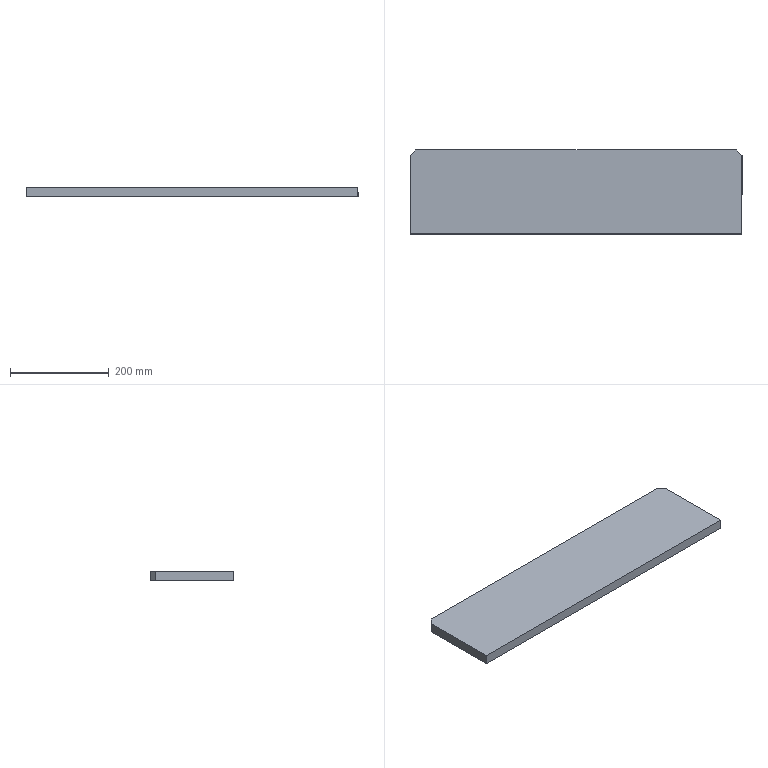Part | SolidWorks | features Chamfer 1, FlatPattern 1, SMBaseFlange 1, SheetMetal 1 | 1 solid | 8 faces | box 672 x 170 x 20 mm | volume 2281920 mm3 | plane 8
STEP:
#1=CARTESIAN_POINT('',(0.,158.,0.));
#2=VERTEX_POINT('',#1);
#3=CARTESIAN_POINT('',(0.,0.,0.));
#4=VERTEX_POINT('',#3);
#5=CARTESIAN_POINT('',(0.,0.,0.));
#6=DIRECTION('',(0.,-1.,0.));
#7=VECTOR('',#6,1000.);
#8=LINE('',#5,#7);
#9=EDGE_CURVE('',#2,#4,#8,.T.);
#10=ORIENTED_EDGE('',*,*,#9,.F.);
#11=CARTESIAN_POINT('',(0.,158.,-20.));
#12=VERTEX_POINT('',#11);
#13=CARTESIAN_POINT('',(0.,158.,-20.));
#14=DIRECTION('',(0.,0.,-1.));
#15=VECTOR('',#14,1000.);
#16=LINE('',#13,#15);
#17=EDGE_CURVE('',#2,#12,#16,.T.);
#18=ORIENTED_EDGE('',*,*,#17,.T.);
#19=CARTESIAN_POINT('',(0.,0.,-20.));
#20=VERTEX_POINT('',#19);
#21=CARTESIAN_POINT('',(0.,0.,-20.));
#22=DIRECTION('',(0.,-1.,0.));
#23=VECTOR('',#22,1000.);
#24=LINE('',#21,#23);
#25=EDGE_CURVE('',#12,#20,#24,.T.);
#26=ORIENTED_EDGE('',*,*,#25,.T.);
#27=CARTESIAN_POINT('',(0.,0.,-20.));
#28=DIRECTION('',(0.,0.,1.));
#29=VECTOR('',#28,1000.);
#30=LINE('',#27,#29);
#31=EDGE_CURVE('',#20,#4,#30,.T.);
#32=ORIENTED_EDGE('',*,*,#31,.T.);
#33=EDGE_LOOP('',(#10,#18,#26,#32));
#34=FACE_OUTER_BOUND('',#33,.T.);
#35=CARTESIAN_POINT('',(0.,0.,-20.));
#36=DIRECTION('',(-1.,0.,0.));
#37=DIRECTION('',(0.,0.,1.));
#38=AXIS2_PLACEMENT_3D('',#35,#36,#37);
#39=PLANE('',#38);
#40=ADVANCED_FACE('',(#34),#39,.T.);
#41=CARTESIAN_POINT('',(660.,170.,0.));
#42=VERTEX_POINT('',#41);
#43=CARTESIAN_POINT('',(12.,170.,0.));
#44=VERTEX_POINT('',#43);
#45=CARTESIAN_POINT('',(0.,170.,0.));
#46=DIRECTION('',(-1.,0.,0.));
#47=VECTOR('',#46,1000.);
#48=LINE('',#45,#47);
#49=EDGE_CURVE('',#42,#44,#48,.T.);
#50=ORIENTED_EDGE('',*,*,#49,.F.);
#51=CARTESIAN_POINT('',(660.,170.,-20.));
#52=VERTEX_POINT('',#51);
#53=CARTESIAN_POINT('',(660.,170.,-20.));
#54=DIRECTION('',(0.,0.,-1.));
#55=VECTOR('',#54,1000.);
#56=LINE('',#53,#55);
#57=EDGE_CURVE('',#42,#52,#56,.T.);
#58=ORIENTED_EDGE('',*,*,#57,.T.);
#59=CARTESIAN_POINT('',(12.,170.,-20.));
#60=VERTEX_POINT('',#59);
#61=CARTESIAN_POINT('',(0.,170.,-20.));
#62=DIRECTION('',(-1.,0.,0.));
#63=VECTOR('',#62,1000.);
#64=LINE('',#61,#63);
#65=EDGE_CURVE('',#52,#60,#64,.T.);
#66=ORIENTED_EDGE('',*,*,#65,.T.);
#67=CARTESIAN_POINT('',(12.,170.,-20.));
#68=DIRECTION('',(0.,0.,1.));
#69=VECTOR('',#68,1000.);
#70=LINE('',#67,#69);
#71=EDGE_CURVE('',#60,#44,#70,.T.);
#72=ORIENTED_EDGE('',*,*,#71,.T.);
#73=EDGE_LOOP('',(#50,#58,#66,#72));
#74=FACE_OUTER_BOUND('',#73,.T.);
#75=CARTESIAN_POINT('',(0.,170.,-20.));
#76=DIRECTION('',(0.,1.,0.));
#77=DIRECTION('',(0.,0.,1.));
#78=AXIS2_PLACEMENT_3D('',#75,#76,#77);
#79=PLANE('',#78);
#80=ADVANCED_FACE('',(#74),#79,.T.);
#81=CARTESIAN_POINT('',(672.,0.,-20.));
#82=VERTEX_POINT('',#81);
#83=CARTESIAN_POINT('',(672.,158.,-20.));
#84=VERTEX_POINT('',#83);
#85=CARTESIAN_POINT('',(672.,0.,-20.));
#86=DIRECTION('',(0.,1.,0.));
#87=VECTOR('',#86,1000.);
#88=LINE('',#85,#87);
#89=EDGE_CURVE('',#82,#84,#88,.T.);
#90=ORIENTED_EDGE('',*,*,#89,.T.);
#91=CARTESIAN_POINT('',(672.,158.,0.));
#92=VERTEX_POINT('',#91);
#93=CARTESIAN_POINT('',(672.,158.,-20.));
#94=DIRECTION('',(0.,0.,1.));
#95=VECTOR('',#94,1000.);
#96=LINE('',#93,#95);
#97=EDGE_CURVE('',#84,#92,#96,.T.);
#98=ORIENTED_EDGE('',*,*,#97,.T.);
#99=CARTESIAN_POINT('',(672.,0.,0.));
#100=VERTEX_POINT('',#99);
#101=CARTESIAN_POINT('',(672.,0.,0.));
#102=DIRECTION('',(0.,1.,0.));
#103=VECTOR('',#102,1000.);
#104=LINE('',#101,#103);
#105=EDGE_CURVE('',#100,#92,#104,.T.);
#106=ORIENTED_EDGE('',*,*,#105,.F.);
#107=CARTESIAN_POINT('',(672.,0.,-20.));
#108=DIRECTION('',(0.,0.,1.));
#109=VECTOR('',#108,1000.);
#110=LINE('',#107,#109);
#111=EDGE_CURVE('',#82,#100,#110,.T.);
#112=ORIENTED_EDGE('',*,*,#111,.F.);
#113=EDGE_LOOP('',(#90,#98,#106,#112));
#114=FACE_OUTER_BOUND('',#113,.T.);
#115=CARTESIAN_POINT('',(672.,0.,-20.));
#116=DIRECTION('',(1.,0.,0.));
#117=DIRECTION('',(0.,0.,-1.));
#118=AXIS2_PLACEMENT_3D('',#115,#116,#117);
#119=PLANE('',#118);
#120=ADVANCED_FACE('',(#114),#119,.T.);
#121=CARTESIAN_POINT('',(0.,0.,0.));
#122=DIRECTION('',(1.,0.,0.));
#123=VECTOR('',#122,1000.);
#124=LINE('',#121,#123);
#125=EDGE_CURVE('',#4,#100,#124,.T.);
#126=ORIENTED_EDGE('',*,*,#125,.F.);
#127=ORIENTED_EDGE('',*,*,#31,.F.);
#128=CARTESIAN_POINT('',(0.,0.,-20.));
#129=DIRECTION('',(1.,0.,0.));
#130=VECTOR('',#129,1000.);
#131=LINE('',#128,#130);
#132=EDGE_CURVE('',#20,#82,#131,.T.);
#133=ORIENTED_EDGE('',*,*,#132,.T.);
#134=ORIENTED_EDGE('',*,*,#111,.T.);
#135=EDGE_LOOP('',(#126,#127,#133,#134));
#136=FACE_OUTER_BOUND('',#135,.T.);
#137=CARTESIAN_POINT('',(0.,0.,-20.));
#138=DIRECTION('',(0.,-1.,0.));
#139=DIRECTION('',(0.,0.,-1.));
#140=AXIS2_PLACEMENT_3D('',#137,#138,#139);
#141=PLANE('',#140);
#142=ADVANCED_FACE('',(#136),#141,.T.);
#143=ORIENTED_EDGE('',*,*,#65,.F.);
#144=CARTESIAN_POINT('',(330.,500.,-20.));
#145=DIRECTION('',(0.7071,-0.7071,0.));
#146=VECTOR('',#145,1000.);
#147=LINE('',#144,#146);
#148=EDGE_CURVE('',#52,#84,#147,.T.);
#149=ORIENTED_EDGE('',*,*,#148,.T.);
#150=ORIENTED_EDGE('',*,*,#89,.F.);
#151=ORIENTED_EDGE('',*,*,#132,.F.);
#152=ORIENTED_EDGE('',*,*,#25,.F.);
#153=CARTESIAN_POINT('',(6.,164.,-20.));
#154=DIRECTION('',(0.7071,0.7071,0.));
#155=VECTOR('',#154,1000.);
#156=LINE('',#153,#155);
#157=EDGE_CURVE('',#12,#60,#156,.T.);
#158=ORIENTED_EDGE('',*,*,#157,.T.);
#159=EDGE_LOOP('',(#143,#149,#150,#151,#152,#158));
#160=FACE_OUTER_BOUND('',#159,.T.);
#161=CARTESIAN_POINT('',(0.,170.,-20.));
#162=DIRECTION('',(0.,0.,-1.));
#163=DIRECTION('',(-1.,0.,0.));
#164=AXIS2_PLACEMENT_3D('',#161,#162,#163);
#165=PLANE('',#164);
#166=ADVANCED_FACE('',(#160),#165,.T.);
#167=ORIENTED_EDGE('',*,*,#105,.T.);
#168=CARTESIAN_POINT('',(672.,158.,0.));
#169=DIRECTION('',(-0.7071,0.7071,0.));
#170=VECTOR('',#169,1000.);
#171=LINE('',#168,#170);
#172=EDGE_CURVE('',#92,#42,#171,.T.);
#173=ORIENTED_EDGE('',*,*,#172,.T.);
#174=ORIENTED_EDGE('',*,*,#49,.T.);
#175=CARTESIAN_POINT('',(12.,170.,0.));
#176=DIRECTION('',(-0.7071,-0.7071,0.));
#177=VECTOR('',#176,1000.);
#178=LINE('',#175,#177);
#179=EDGE_CURVE('',#44,#2,#178,.T.);
#180=ORIENTED_EDGE('',*,*,#179,.T.);
#181=ORIENTED_EDGE('',*,*,#9,.T.);
#182=ORIENTED_EDGE('',*,*,#125,.T.);
#183=EDGE_LOOP('',(#167,#173,#174,#180,#181,#182));
#184=FACE_OUTER_BOUND('',#183,.T.);
#185=CARTESIAN_POINT('',(0.,170.,0.));
#186=DIRECTION('',(0.,0.,-1.));
#187=DIRECTION('',(-1.,0.,0.));
#188=AXIS2_PLACEMENT_3D('',#185,#186,#187);
#189=PLANE('',#188);
#190=ADVANCED_FACE('',(#184),#189,.F.);
#191=ORIENTED_EDGE('',*,*,#148,.F.);
#192=ORIENTED_EDGE('',*,*,#57,.F.);
#193=ORIENTED_EDGE('',*,*,#172,.F.);
#194=ORIENTED_EDGE('',*,*,#97,.F.);
#195=EDGE_LOOP('',(#191,#192,#193,#194));
#196=FACE_OUTER_BOUND('',#195,.T.);
#197=CARTESIAN_POINT('',(672.,158.,-20.));
#198=DIRECTION('',(-0.7071,-0.7071,0.));
#199=DIRECTION('',(0.7071,-0.7071,0.));
#200=AXIS2_PLACEMENT_3D('',#197,#198,#199);
#201=PLANE('',#200);
#202=ADVANCED_FACE('',(#196),#201,.F.);
#203=ORIENTED_EDGE('',*,*,#157,.F.);
#204=ORIENTED_EDGE('',*,*,#17,.F.);
#205=ORIENTED_EDGE('',*,*,#179,.F.);
#206=ORIENTED_EDGE('',*,*,#71,.F.);
#207=EDGE_LOOP('',(#203,#204,#205,#206));
#208=FACE_OUTER_BOUND('',#207,.T.);
#209=CARTESIAN_POINT('',(12.,170.,-20.));
#210=DIRECTION('',(0.7071,-0.7071,0.));
#211=DIRECTION('',(0.7071,0.7071,0.));
#212=AXIS2_PLACEMENT_3D('',#209,#210,#211);
#213=PLANE('',#212);
#214=ADVANCED_FACE('',(#208),#213,.F.);
#215=CLOSED_SHELL('',(#40,#80,#120,#142,#166,#190,#202,#214));
#216=MANIFOLD_SOLID_BREP('',#215);
#217=CARTESIAN_POINT('',(0.,0.,0.));
#218=DIRECTION('',(0.,0.,1.));
#219=DIRECTION('',(1.,0.,0.));
#220=AXIS2_PLACEMENT_3D('',#217,#218,#219);
#221=(LENGTH_UNIT()NAMED_UNIT(*)SI_UNIT(.MILLI.,.METRE.));
#222=UNCERTAINTY_MEASURE_WITH_UNIT(LENGTH_MEASURE(0.00001),#221,'','');
#223=(NAMED_UNIT(*)PLANE_ANGLE_UNIT()SI_UNIT($,.RADIAN.));
#224=(NAMED_UNIT(*)SI_UNIT($,.STERADIAN.)SOLID_ANGLE_UNIT());
#225=(GEOMETRIC_REPRESENTATION_CONTEXT(3)GLOBAL_UNCERTAINTY_ASSIGNED_CONTEXT((#222))GLOBAL_UNIT_ASSIGNED_CONTEXT((#221,#223,#224))REPRESENTATION_CONTEXT('',''));
#226=ADVANCED_BREP_SHAPE_REPRESENTATION('',(#216,#220),#225);